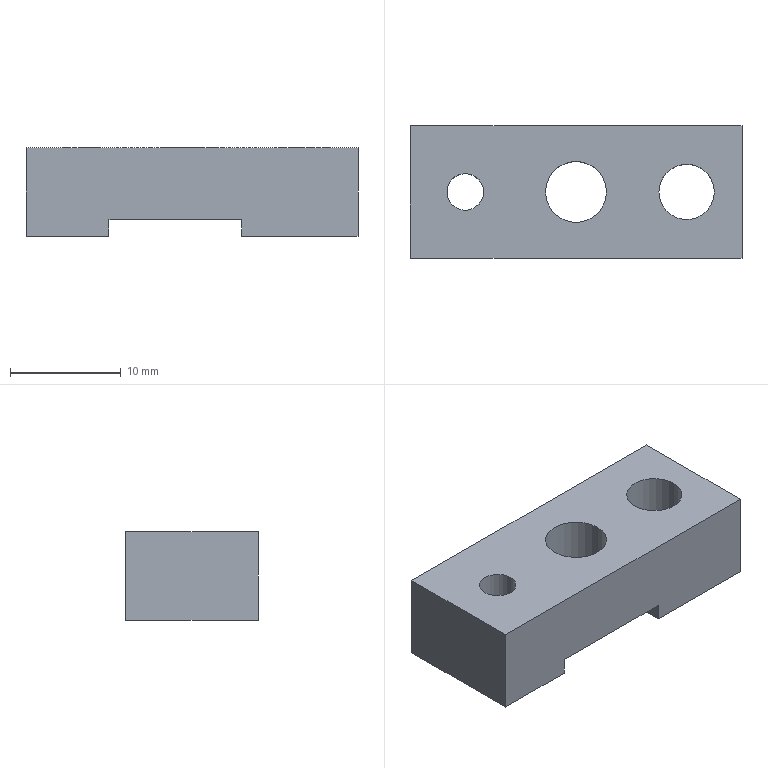Part | NX | features BREP 1 | 1 solid | 16 faces | box 30 x 12 x 8 mm | volume 2284 mm3 | plane 10 | cylinder 6 | commonest cylinder face diameters 3.3 x2 5 x2 5.5 x2
STEP:
#1=CARTESIAN_POINT('',(-768.139,-6.,1.5));
#2=VERTEX_POINT('',#1);
#3=CARTESIAN_POINT('',(-762.639,-6.,1.5));
#4=VERTEX_POINT('',#3);
#5=CARTESIAN_POINT('',(-765.389,-6.,1.5));
#6=DIRECTION('',(0.,0.,1.));
#7=DIRECTION('',(1.,0.,0.));
#8=AXIS2_PLACEMENT_3D('',#5,#6,#7);
#9=CIRCLE('',#8,2.75);
#10=EDGE_CURVE('',#2,#4,#9,.T.);
#11=ORIENTED_EDGE('',*,*,#10,.F.);
#12=CARTESIAN_POINT('',(-768.139,-6.,8.));
#13=VERTEX_POINT('',#12);
#14=CARTESIAN_POINT('',(-768.139,-6.,0.));
#15=DIRECTION('',(0.,0.,1.));
#16=VECTOR('',#15,1000.);
#17=LINE('',#14,#16);
#18=EDGE_CURVE('',#13,#2,#17,.F.);
#19=ORIENTED_EDGE('',*,*,#18,.F.);
#20=CARTESIAN_POINT('',(-762.639,-6.,8.));
#21=VERTEX_POINT('',#20);
#22=CARTESIAN_POINT('',(-765.389,-6.,8.));
#23=DIRECTION('',(0.,0.,1.));
#24=DIRECTION('',(1.,0.,0.));
#25=AXIS2_PLACEMENT_3D('',#22,#23,#24);
#26=CIRCLE('',#25,2.75);
#27=EDGE_CURVE('',#13,#21,#26,.T.);
#28=ORIENTED_EDGE('',*,*,#27,.T.);
#29=CARTESIAN_POINT('',(-762.639,-6.,0.));
#30=DIRECTION('',(0.,0.,1.));
#31=VECTOR('',#30,1000.);
#32=LINE('',#29,#31);
#33=EDGE_CURVE('',#21,#4,#32,.F.);
#34=ORIENTED_EDGE('',*,*,#33,.T.);
#35=EDGE_LOOP('',(#11,#19,#28,#34));
#36=FACE_BOUND('',#35,.T.);
#37=CARTESIAN_POINT('',(-765.389,-6.,0.));
#38=DIRECTION('',(0.,0.,1.));
#39=DIRECTION('',(1.,0.,0.));
#40=AXIS2_PLACEMENT_3D('',#37,#38,#39);
#41=CYLINDRICAL_SURFACE('',#40,2.75);
#42=ADVANCED_FACE('',(#36),#41,.F.);
#43=CARTESIAN_POINT('',(-773.739,-6.,8.));
#44=VERTEX_POINT('',#43);
#45=CARTESIAN_POINT('',(-777.039,-6.,8.));
#46=VERTEX_POINT('',#45);
#47=CARTESIAN_POINT('',(-775.389,-6.,8.));
#48=DIRECTION('',(0.,0.,-1.));
#49=DIRECTION('',(-1.,0.,0.));
#50=AXIS2_PLACEMENT_3D('',#47,#48,#49);
#51=CIRCLE('',#50,1.65);
#52=EDGE_CURVE('',#44,#46,#51,.T.);
#53=ORIENTED_EDGE('',*,*,#52,.F.);
#54=CARTESIAN_POINT('',(-773.739,-6.,0.));
#55=VERTEX_POINT('',#54);
#56=CARTESIAN_POINT('',(-773.739,-6.,0.));
#57=DIRECTION('',(0.,0.,-1.));
#58=VECTOR('',#57,1000.);
#59=LINE('',#56,#58);
#60=EDGE_CURVE('',#44,#55,#59,.T.);
#61=ORIENTED_EDGE('',*,*,#60,.T.);
#62=CARTESIAN_POINT('',(-777.039,-6.,0.));
#63=VERTEX_POINT('',#62);
#64=CARTESIAN_POINT('',(-775.389,-6.,0.));
#65=DIRECTION('',(0.,0.,-1.));
#66=DIRECTION('',(-1.,0.,0.));
#67=AXIS2_PLACEMENT_3D('',#64,#65,#66);
#68=CIRCLE('',#67,1.65);
#69=EDGE_CURVE('',#55,#63,#68,.T.);
#70=ORIENTED_EDGE('',*,*,#69,.T.);
#71=CARTESIAN_POINT('',(-777.039,-6.,0.));
#72=DIRECTION('',(0.,0.,-1.));
#73=VECTOR('',#72,1000.);
#74=LINE('',#71,#73);
#75=EDGE_CURVE('',#46,#63,#74,.T.);
#76=ORIENTED_EDGE('',*,*,#75,.F.);
#77=EDGE_LOOP('',(#53,#61,#70,#76));
#78=FACE_BOUND('',#77,.T.);
#79=CARTESIAN_POINT('',(-775.389,-6.,0.));
#80=DIRECTION('',(0.,0.,-1.));
#81=DIRECTION('',(-1.,0.,0.));
#82=AXIS2_PLACEMENT_3D('',#79,#80,#81);
#83=CYLINDRICAL_SURFACE('',#82,1.65);
#84=ADVANCED_FACE('',(#78),#83,.F.);
#85=CARTESIAN_POINT('',(-752.889,-6.,8.));
#86=VERTEX_POINT('',#85);
#87=CARTESIAN_POINT('',(-757.889,-6.,8.));
#88=VERTEX_POINT('',#87);
#89=CARTESIAN_POINT('',(-755.389,-6.,8.));
#90=DIRECTION('',(0.,0.,-1.));
#91=DIRECTION('',(-1.,0.,0.));
#92=AXIS2_PLACEMENT_3D('',#89,#90,#91);
#93=CIRCLE('',#92,2.5);
#94=EDGE_CURVE('',#86,#88,#93,.T.);
#95=ORIENTED_EDGE('',*,*,#94,.F.);
#96=CARTESIAN_POINT('',(-752.889,-6.,0.));
#97=VERTEX_POINT('',#96);
#98=CARTESIAN_POINT('',(-752.889,-6.,0.));
#99=DIRECTION('',(0.,0.,-1.));
#100=VECTOR('',#99,1000.);
#101=LINE('',#98,#100);
#102=EDGE_CURVE('',#86,#97,#101,.T.);
#103=ORIENTED_EDGE('',*,*,#102,.T.);
#104=CARTESIAN_POINT('',(-757.889,-6.,0.));
#105=VERTEX_POINT('',#104);
#106=CARTESIAN_POINT('',(-755.389,-6.,0.));
#107=DIRECTION('',(0.,0.,-1.));
#108=DIRECTION('',(-1.,0.,0.));
#109=AXIS2_PLACEMENT_3D('',#106,#107,#108);
#110=CIRCLE('',#109,2.5);
#111=EDGE_CURVE('',#97,#105,#110,.T.);
#112=ORIENTED_EDGE('',*,*,#111,.T.);
#113=CARTESIAN_POINT('',(-757.889,-6.,0.));
#114=DIRECTION('',(0.,0.,-1.));
#115=VECTOR('',#114,1000.);
#116=LINE('',#113,#115);
#117=EDGE_CURVE('',#88,#105,#116,.T.);
#118=ORIENTED_EDGE('',*,*,#117,.F.);
#119=EDGE_LOOP('',(#95,#103,#112,#118));
#120=FACE_BOUND('',#119,.T.);
#121=CARTESIAN_POINT('',(-755.389,-6.,0.));
#122=DIRECTION('',(0.,0.,-1.));
#123=DIRECTION('',(-1.,0.,0.));
#124=AXIS2_PLACEMENT_3D('',#121,#122,#123);
#125=CYLINDRICAL_SURFACE('',#124,2.5);
#126=ADVANCED_FACE('',(#120),#125,.F.);
#127=CARTESIAN_POINT('',(-760.889,-12.,0.));
#128=VERTEX_POINT('',#127);
#129=CARTESIAN_POINT('',(-750.389,-12.,0.));
#130=VERTEX_POINT('',#129);
#131=CARTESIAN_POINT('',(-750.389,-12.,0.));
#132=DIRECTION('',(1.,0.,0.));
#133=VECTOR('',#132,1000.);
#134=LINE('',#131,#133);
#135=EDGE_CURVE('',#128,#130,#134,.T.);
#136=ORIENTED_EDGE('',*,*,#135,.F.);
#137=CARTESIAN_POINT('',(-760.889,0.,0.));
#138=VERTEX_POINT('',#137);
#139=CARTESIAN_POINT('',(-760.889,0.,0.));
#140=DIRECTION('',(0.,-1.,0.));
#141=VECTOR('',#140,1000.);
#142=LINE('',#139,#141);
#143=EDGE_CURVE('',#138,#128,#142,.T.);
#144=ORIENTED_EDGE('',*,*,#143,.F.);
#145=CARTESIAN_POINT('',(-750.389,0.,0.));
#146=VERTEX_POINT('',#145);
#147=CARTESIAN_POINT('',(-750.389,0.,0.));
#148=DIRECTION('',(-1.,0.,0.));
#149=VECTOR('',#148,1000.);
#150=LINE('',#147,#149);
#151=EDGE_CURVE('',#146,#138,#150,.T.);
#152=ORIENTED_EDGE('',*,*,#151,.F.);
#153=CARTESIAN_POINT('',(-750.389,-12.,0.));
#154=DIRECTION('',(0.,1.,0.));
#155=VECTOR('',#154,1000.);
#156=LINE('',#153,#155);
#157=EDGE_CURVE('',#130,#146,#156,.T.);
#158=ORIENTED_EDGE('',*,*,#157,.F.);
#159=EDGE_LOOP('',(#136,#144,#152,#158));
#160=FACE_BOUND('',#159,.T.);
#161=CARTESIAN_POINT('',(-755.389,-6.,0.));
#162=DIRECTION('',(0.,0.,-1.));
#163=DIRECTION('',(-1.,0.,0.));
#164=AXIS2_PLACEMENT_3D('',#161,#162,#163);
#165=CIRCLE('',#164,2.5);
#166=EDGE_CURVE('',#105,#97,#165,.T.);
#167=ORIENTED_EDGE('',*,*,#166,.F.);
#168=ORIENTED_EDGE('',*,*,#111,.F.);
#169=EDGE_LOOP('',(#167,#168));
#170=FACE_BOUND('',#169,.T.);
#171=CARTESIAN_POINT('',(-750.389,0.,0.));
#172=DIRECTION('',(0.,0.,1.));
#173=DIRECTION('',(1.,0.,0.));
#174=AXIS2_PLACEMENT_3D('',#171,#172,#173);
#175=PLANE('',#174);
#176=ADVANCED_FACE('',(#160,#170),#175,.F.);
#177=ORIENTED_EDGE('',*,*,#157,.T.);
#178=CARTESIAN_POINT('',(-750.389,0.,8.));
#179=VERTEX_POINT('',#178);
#180=CARTESIAN_POINT('',(-750.389,0.,8.));
#181=DIRECTION('',(0.,0.,-1.));
#182=VECTOR('',#181,1000.);
#183=LINE('',#180,#182);
#184=EDGE_CURVE('',#179,#146,#183,.T.);
#185=ORIENTED_EDGE('',*,*,#184,.F.);
#186=CARTESIAN_POINT('',(-750.389,-12.,8.));
#187=VERTEX_POINT('',#186);
#188=CARTESIAN_POINT('',(-750.389,-12.,8.));
#189=DIRECTION('',(0.,1.,0.));
#190=VECTOR('',#189,1000.);
#191=LINE('',#188,#190);
#192=EDGE_CURVE('',#187,#179,#191,.T.);
#193=ORIENTED_EDGE('',*,*,#192,.F.);
#194=CARTESIAN_POINT('',(-750.389,-12.,8.));
#195=DIRECTION('',(0.,0.,-1.));
#196=VECTOR('',#195,1000.);
#197=LINE('',#194,#196);
#198=EDGE_CURVE('',#187,#130,#197,.T.);
#199=ORIENTED_EDGE('',*,*,#198,.T.);
#200=EDGE_LOOP('',(#177,#185,#193,#199));
#201=FACE_BOUND('',#200,.T.);
#202=CARTESIAN_POINT('',(-750.389,-12.,8.));
#203=DIRECTION('',(-1.,0.,0.));
#204=DIRECTION('',(0.,0.,1.));
#205=AXIS2_PLACEMENT_3D('',#202,#203,#204);
#206=PLANE('',#205);
#207=ADVANCED_FACE('',(#201),#206,.F.);
#208=ORIENTED_EDGE('',*,*,#151,.T.);
#209=CARTESIAN_POINT('',(-760.889,0.,1.5));
#210=VERTEX_POINT('',#209);
#211=CARTESIAN_POINT('',(-760.889,0.,0.));
#212=DIRECTION('',(0.,0.,1.));
#213=VECTOR('',#212,1000.);
#214=LINE('',#211,#213);
#215=EDGE_CURVE('',#138,#210,#214,.T.);
#216=ORIENTED_EDGE('',*,*,#215,.T.);
#217=CARTESIAN_POINT('',(-772.889,0.,1.5));
#218=VERTEX_POINT('',#217);
#219=CARTESIAN_POINT('',(-760.889,0.,1.5));
#220=DIRECTION('',(-1.,0.,0.));
#221=VECTOR('',#220,1000.);
#222=LINE('',#219,#221);
#223=EDGE_CURVE('',#210,#218,#222,.T.);
#224=ORIENTED_EDGE('',*,*,#223,.T.);
#225=CARTESIAN_POINT('',(-772.889,0.,0.));
#226=VERTEX_POINT('',#225);
#227=CARTESIAN_POINT('',(-772.889,0.,0.));
#228=DIRECTION('',(0.,0.,-1.));
#229=VECTOR('',#228,1000.);
#230=LINE('',#227,#229);
#231=EDGE_CURVE('',#218,#226,#230,.T.);
#232=ORIENTED_EDGE('',*,*,#231,.T.);
#233=CARTESIAN_POINT('',(-780.389,0.,0.));
#234=VERTEX_POINT('',#233);
#235=CARTESIAN_POINT('',(-750.389,0.,0.));
#236=DIRECTION('',(-1.,0.,0.));
#237=VECTOR('',#236,1000.);
#238=LINE('',#235,#237);
#239=EDGE_CURVE('',#226,#234,#238,.T.);
#240=ORIENTED_EDGE('',*,*,#239,.T.);
#241=CARTESIAN_POINT('',(-780.389,0.,8.));
#242=VERTEX_POINT('',#241);
#243=CARTESIAN_POINT('',(-780.389,0.,8.));
#244=DIRECTION('',(0.,0.,-1.));
#245=VECTOR('',#244,1000.);
#246=LINE('',#243,#245);
#247=EDGE_CURVE('',#242,#234,#246,.T.);
#248=ORIENTED_EDGE('',*,*,#247,.F.);
#249=CARTESIAN_POINT('',(-750.389,0.,8.));
#250=DIRECTION('',(-1.,0.,0.));
#251=VECTOR('',#250,1000.);
#252=LINE('',#249,#251);
#253=EDGE_CURVE('',#179,#242,#252,.T.);
#254=ORIENTED_EDGE('',*,*,#253,.F.);
#255=ORIENTED_EDGE('',*,*,#184,.T.);
#256=EDGE_LOOP('',(#208,#216,#224,#232,#240,#248,#254,#255));
#257=FACE_BOUND('',#256,.T.);
#258=CARTESIAN_POINT('',(-750.389,0.,8.));
#259=DIRECTION('',(0.,-1.,0.));
#260=DIRECTION('',(0.,0.,-1.));
#261=AXIS2_PLACEMENT_3D('',#258,#259,#260);
#262=PLANE('',#261);
#263=ADVANCED_FACE('',(#257),#262,.F.);
#264=CARTESIAN_POINT('',(-780.389,-12.,0.));
#265=VERTEX_POINT('',#264);
#266=CARTESIAN_POINT('',(-780.389,-12.,0.));
#267=DIRECTION('',(0.,-1.,0.));
#268=VECTOR('',#267,1000.);
#269=LINE('',#266,#268);
#270=EDGE_CURVE('',#234,#265,#269,.T.);
#271=ORIENTED_EDGE('',*,*,#270,.T.);
#272=CARTESIAN_POINT('',(-780.389,-12.,8.));
#273=VERTEX_POINT('',#272);
#274=CARTESIAN_POINT('',(-780.389,-12.,8.));
#275=DIRECTION('',(0.,0.,-1.));
#276=VECTOR('',#275,1000.);
#277=LINE('',#274,#276);
#278=EDGE_CURVE('',#273,#265,#277,.T.);
#279=ORIENTED_EDGE('',*,*,#278,.F.);
#280=CARTESIAN_POINT('',(-780.389,-12.,8.));
#281=DIRECTION('',(0.,-1.,0.));
#282=VECTOR('',#281,1000.);
#283=LINE('',#280,#282);
#284=EDGE_CURVE('',#242,#273,#283,.T.);
#285=ORIENTED_EDGE('',*,*,#284,.F.);
#286=ORIENTED_EDGE('',*,*,#247,.T.);
#287=EDGE_LOOP('',(#271,#279,#285,#286));
#288=FACE_BOUND('',#287,.T.);
#289=CARTESIAN_POINT('',(-780.389,-12.,8.));
#290=DIRECTION('',(1.,0.,0.));
#291=DIRECTION('',(0.,1.,0.));
#292=AXIS2_PLACEMENT_3D('',#289,#290,#291);
#293=PLANE('',#292);
#294=ADVANCED_FACE('',(#288),#293,.F.);
#295=CARTESIAN_POINT('',(-760.889,-12.,1.5));
#296=VERTEX_POINT('',#295);
#297=CARTESIAN_POINT('',(-772.889,-12.,1.5));
#298=VERTEX_POINT('',#297);
#299=CARTESIAN_POINT('',(-760.889,-12.,1.5));
#300=DIRECTION('',(-1.,0.,0.));
#301=VECTOR('',#300,1000.);
#302=LINE('',#299,#301);
#303=EDGE_CURVE('',#296,#298,#302,.T.);
#304=ORIENTED_EDGE('',*,*,#303,.F.);
#305=CARTESIAN_POINT('',(-760.889,-12.,0.));
#306=DIRECTION('',(0.,0.,1.));
#307=VECTOR('',#306,1000.);
#308=LINE('',#305,#307);
#309=EDGE_CURVE('',#128,#296,#308,.T.);
#310=ORIENTED_EDGE('',*,*,#309,.F.);
#311=ORIENTED_EDGE('',*,*,#135,.T.);
#312=ORIENTED_EDGE('',*,*,#198,.F.);
#313=CARTESIAN_POINT('',(-750.389,-12.,8.));
#314=DIRECTION('',(1.,0.,0.));
#315=VECTOR('',#314,1000.);
#316=LINE('',#313,#315);
#317=EDGE_CURVE('',#273,#187,#316,.T.);
#318=ORIENTED_EDGE('',*,*,#317,.F.);
#319=ORIENTED_EDGE('',*,*,#278,.T.);
#320=CARTESIAN_POINT('',(-772.889,-12.,0.));
#321=VERTEX_POINT('',#320);
#322=CARTESIAN_POINT('',(-750.389,-12.,0.));
#323=DIRECTION('',(1.,0.,0.));
#324=VECTOR('',#323,1000.);
#325=LINE('',#322,#324);
#326=EDGE_CURVE('',#265,#321,#325,.T.);
#327=ORIENTED_EDGE('',*,*,#326,.T.);
#328=CARTESIAN_POINT('',(-772.889,-12.,0.));
#329=DIRECTION('',(0.,0.,-1.));
#330=VECTOR('',#329,1000.);
#331=LINE('',#328,#330);
#332=EDGE_CURVE('',#298,#321,#331,.T.);
#333=ORIENTED_EDGE('',*,*,#332,.F.);
#334=EDGE_LOOP('',(#304,#310,#311,#312,#318,#319,#327,#333));
#335=FACE_BOUND('',#334,.T.);
#336=CARTESIAN_POINT('',(-750.389,-12.,8.));
#337=DIRECTION('',(0.,1.,0.));
#338=DIRECTION('',(1.,0.,0.));
#339=AXIS2_PLACEMENT_3D('',#336,#337,#338);
#340=PLANE('',#339);
#341=ADVANCED_FACE('',(#335),#340,.F.);
#342=ORIENTED_EDGE('',*,*,#192,.T.);
#343=ORIENTED_EDGE('',*,*,#253,.T.);
#344=ORIENTED_EDGE('',*,*,#284,.T.);
#345=ORIENTED_EDGE('',*,*,#317,.T.);
#346=EDGE_LOOP('',(#342,#343,#344,#345));
#347=FACE_BOUND('',#346,.T.);
#348=CARTESIAN_POINT('',(-765.389,-6.,8.));
#349=DIRECTION('',(0.,0.,1.));
#350=DIRECTION('',(1.,0.,0.));
#351=AXIS2_PLACEMENT_3D('',#348,#349,#350);
#352=CIRCLE('',#351,2.75);
#353=EDGE_CURVE('',#21,#13,#352,.T.);
#354=ORIENTED_EDGE('',*,*,#353,.F.);
#355=ORIENTED_EDGE('',*,*,#27,.F.);
#356=EDGE_LOOP('',(#354,#355));
#357=FACE_BOUND('',#356,.T.);
#358=CARTESIAN_POINT('',(-775.389,-6.,8.));
#359=DIRECTION('',(0.,0.,-1.));
#360=DIRECTION('',(-1.,0.,0.));
#361=AXIS2_PLACEMENT_3D('',#358,#359,#360);
#362=CIRCLE('',#361,1.65);
#363=EDGE_CURVE('',#46,#44,#362,.T.);
#364=ORIENTED_EDGE('',*,*,#363,.T.);
#365=ORIENTED_EDGE('',*,*,#52,.T.);
#366=EDGE_LOOP('',(#364,#365));
#367=FACE_BOUND('',#366,.T.);
#368=CARTESIAN_POINT('',(-755.389,-6.,8.));
#369=DIRECTION('',(0.,0.,-1.));
#370=DIRECTION('',(-1.,0.,0.));
#371=AXIS2_PLACEMENT_3D('',#368,#369,#370);
#372=CIRCLE('',#371,2.5);
#373=EDGE_CURVE('',#88,#86,#372,.T.);
#374=ORIENTED_EDGE('',*,*,#373,.T.);
#375=ORIENTED_EDGE('',*,*,#94,.T.);
#376=EDGE_LOOP('',(#374,#375));
#377=FACE_BOUND('',#376,.T.);
#378=CARTESIAN_POINT('',(-750.389,0.,8.));
#379=DIRECTION('',(0.,0.,1.));
#380=DIRECTION('',(1.,0.,0.));
#381=AXIS2_PLACEMENT_3D('',#378,#379,#380);
#382=PLANE('',#381);
#383=ADVANCED_FACE('',(#347,#357,#367,#377),#382,.T.);
#384=ORIENTED_EDGE('',*,*,#239,.F.);
#385=CARTESIAN_POINT('',(-772.889,0.,0.));
#386=DIRECTION('',(0.,-1.,0.));
#387=VECTOR('',#386,1000.);
#388=LINE('',#385,#387);
#389=EDGE_CURVE('',#226,#321,#388,.T.);
#390=ORIENTED_EDGE('',*,*,#389,.T.);
#391=ORIENTED_EDGE('',*,*,#326,.F.);
#392=ORIENTED_EDGE('',*,*,#270,.F.);
#393=EDGE_LOOP('',(#384,#390,#391,#392));
#394=FACE_BOUND('',#393,.T.);
#395=CARTESIAN_POINT('',(-775.389,-6.,0.));
#396=DIRECTION('',(0.,0.,-1.));
#397=DIRECTION('',(-1.,0.,0.));
#398=AXIS2_PLACEMENT_3D('',#395,#396,#397);
#399=CIRCLE('',#398,1.65);
#400=EDGE_CURVE('',#63,#55,#399,.T.);
#401=ORIENTED_EDGE('',*,*,#400,.F.);
#402=ORIENTED_EDGE('',*,*,#69,.F.);
#403=EDGE_LOOP('',(#401,#402));
#404=FACE_BOUND('',#403,.T.);
#405=CARTESIAN_POINT('',(-750.389,0.,0.));
#406=DIRECTION('',(0.,0.,1.));
#407=DIRECTION('',(1.,0.,0.));
#408=AXIS2_PLACEMENT_3D('',#405,#406,#407);
#409=PLANE('',#408);
#410=ADVANCED_FACE('',(#394,#404),#409,.F.);
#411=ORIENTED_EDGE('',*,*,#309,.T.);
#412=CARTESIAN_POINT('',(-760.889,0.,1.5));
#413=DIRECTION('',(0.,-1.,0.));
#414=VECTOR('',#413,1000.);
#415=LINE('',#412,#414);
#416=EDGE_CURVE('',#210,#296,#415,.T.);
#417=ORIENTED_EDGE('',*,*,#416,.F.);
#418=ORIENTED_EDGE('',*,*,#215,.F.);
#419=ORIENTED_EDGE('',*,*,#143,.T.);
#420=EDGE_LOOP('',(#411,#417,#418,#419));
#421=FACE_BOUND('',#420,.T.);
#422=CARTESIAN_POINT('',(-760.889,0.,0.));
#423=DIRECTION('',(1.,0.,0.));
#424=DIRECTION('',(0.,1.,0.));
#425=AXIS2_PLACEMENT_3D('',#422,#423,#424);
#426=PLANE('',#425);
#427=ADVANCED_FACE('',(#421),#426,.F.);
#428=ORIENTED_EDGE('',*,*,#332,.T.);
#429=ORIENTED_EDGE('',*,*,#389,.F.);
#430=ORIENTED_EDGE('',*,*,#231,.F.);
#431=CARTESIAN_POINT('',(-772.889,0.,1.5));
#432=DIRECTION('',(0.,-1.,0.));
#433=VECTOR('',#432,1000.);
#434=LINE('',#431,#433);
#435=EDGE_CURVE('',#218,#298,#434,.T.);
#436=ORIENTED_EDGE('',*,*,#435,.T.);
#437=EDGE_LOOP('',(#428,#429,#430,#436));
#438=FACE_BOUND('',#437,.T.);
#439=CARTESIAN_POINT('',(-772.889,0.,0.));
#440=DIRECTION('',(-1.,0.,0.));
#441=DIRECTION('',(0.,1.,0.));
#442=AXIS2_PLACEMENT_3D('',#439,#440,#441);
#443=PLANE('',#442);
#444=ADVANCED_FACE('',(#438),#443,.F.);
#445=ORIENTED_EDGE('',*,*,#303,.T.);
#446=ORIENTED_EDGE('',*,*,#435,.F.);
#447=ORIENTED_EDGE('',*,*,#223,.F.);
#448=ORIENTED_EDGE('',*,*,#416,.T.);
#449=EDGE_LOOP('',(#445,#446,#447,#448));
#450=FACE_BOUND('',#449,.T.);
#451=CARTESIAN_POINT('',(-765.389,-6.,1.5));
#452=DIRECTION('',(0.,0.,1.));
#453=DIRECTION('',(1.,0.,0.));
#454=AXIS2_PLACEMENT_3D('',#451,#452,#453);
#455=CIRCLE('',#454,2.75);
#456=EDGE_CURVE('',#4,#2,#455,.T.);
#457=ORIENTED_EDGE('',*,*,#456,.T.);
#458=ORIENTED_EDGE('',*,*,#10,.T.);
#459=EDGE_LOOP('',(#457,#458));
#460=FACE_BOUND('',#459,.T.);
#461=CARTESIAN_POINT('',(-760.889,0.,1.5));
#462=DIRECTION('',(0.,0.,1.));
#463=DIRECTION('',(1.,0.,0.));
#464=AXIS2_PLACEMENT_3D('',#461,#462,#463);
#465=PLANE('',#464);
#466=ADVANCED_FACE('',(#450,#460),#465,.F.);
#467=ORIENTED_EDGE('',*,*,#102,.F.);
#468=ORIENTED_EDGE('',*,*,#373,.F.);
#469=ORIENTED_EDGE('',*,*,#117,.T.);
#470=ORIENTED_EDGE('',*,*,#166,.T.);
#471=EDGE_LOOP('',(#467,#468,#469,#470));
#472=FACE_BOUND('',#471,.T.);
#473=CARTESIAN_POINT('',(-755.389,-6.,0.));
#474=DIRECTION('',(0.,0.,-1.));
#475=DIRECTION('',(-1.,0.,0.));
#476=AXIS2_PLACEMENT_3D('',#473,#474,#475);
#477=CYLINDRICAL_SURFACE('',#476,2.5);
#478=ADVANCED_FACE('',(#472),#477,.F.);
#479=ORIENTED_EDGE('',*,*,#60,.F.);
#480=ORIENTED_EDGE('',*,*,#363,.F.);
#481=ORIENTED_EDGE('',*,*,#75,.T.);
#482=ORIENTED_EDGE('',*,*,#400,.T.);
#483=EDGE_LOOP('',(#479,#480,#481,#482));
#484=FACE_BOUND('',#483,.T.);
#485=CARTESIAN_POINT('',(-775.389,-6.,0.));
#486=DIRECTION('',(0.,0.,-1.));
#487=DIRECTION('',(-1.,0.,0.));
#488=AXIS2_PLACEMENT_3D('',#485,#486,#487);
#489=CYLINDRICAL_SURFACE('',#488,1.65);
#490=ADVANCED_FACE('',(#484),#489,.F.);
#491=ORIENTED_EDGE('',*,*,#18,.T.);
#492=ORIENTED_EDGE('',*,*,#456,.F.);
#493=ORIENTED_EDGE('',*,*,#33,.F.);
#494=ORIENTED_EDGE('',*,*,#353,.T.);
#495=EDGE_LOOP('',(#491,#492,#493,#494));
#496=FACE_BOUND('',#495,.T.);
#497=CARTESIAN_POINT('',(-765.389,-6.,0.));
#498=DIRECTION('',(0.,0.,1.));
#499=DIRECTION('',(1.,0.,0.));
#500=AXIS2_PLACEMENT_3D('',#497,#498,#499);
#501=CYLINDRICAL_SURFACE('',#500,2.75);
#502=ADVANCED_FACE('',(#496),#501,.F.);
#503=CLOSED_SHELL('',(#42,#84,#126,#176,#207,#263,#294,#341,#383,#410,#427,#444,#466,#478,#490,#502));
#504=MANIFOLD_SOLID_BREP('',#503);
#505=(LENGTH_UNIT()NAMED_UNIT(*)SI_UNIT(.MILLI.,.METRE.));
#506=UNCERTAINTY_MEASURE_WITH_UNIT(LENGTH_MEASURE(0.00001),#505,'','');
#507=(NAMED_UNIT(*)PLANE_ANGLE_UNIT()SI_UNIT($,.RADIAN.));
#508=(NAMED_UNIT(*)SI_UNIT($,.STERADIAN.)SOLID_ANGLE_UNIT());
#509=(GEOMETRIC_REPRESENTATION_CONTEXT(3)GLOBAL_UNCERTAINTY_ASSIGNED_CONTEXT((#506))GLOBAL_UNIT_ASSIGNED_CONTEXT((#505,#507,#508))REPRESENTATION_CONTEXT('',''));
#510=ADVANCED_BREP_SHAPE_REPRESENTATION('',(#504),#509);